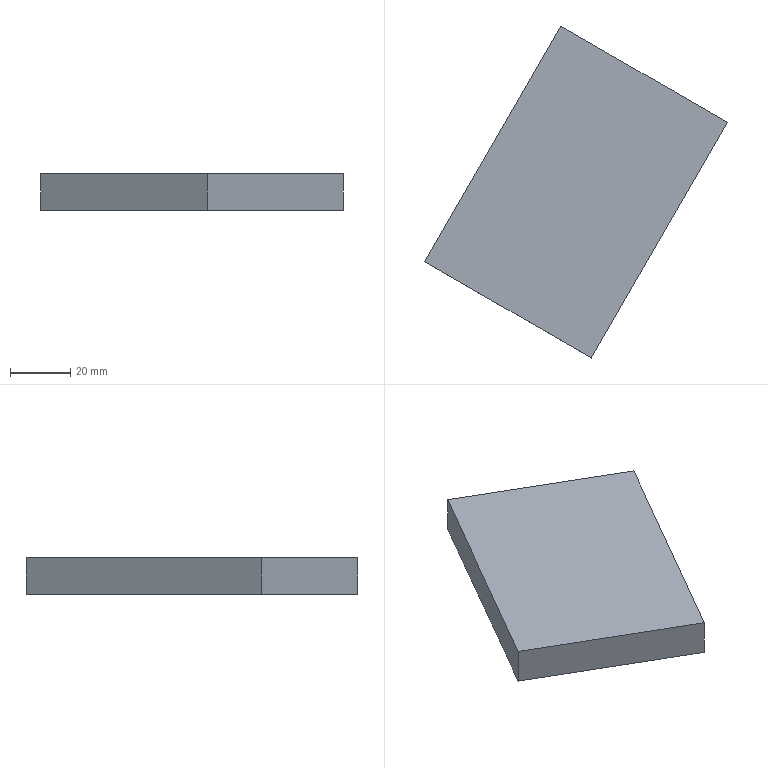Part | SolidWorks | features BaseBody 1 | 1 solid | 6 faces | box 100.197 x 109.81 x 12 mm | volume 68834 mm3 | plane 6
STEP:
#1=CARTESIAN_POINT('',(-225.308,1702.18,-1143.));
#2=VERTEX_POINT('',#1);
#3=CARTESIAN_POINT('',(-280.504,1734.048,-1143.));
#4=VERTEX_POINT('',#3);
#5=CARTESIAN_POINT('',(-225.308,1702.18,-1143.));
#6=DIRECTION('',(-0.866,0.5,0.));
#7=VECTOR('',#6,1000.);
#8=LINE('',#5,#7);
#9=EDGE_CURVE('',#2,#4,#8,.T.);
#10=ORIENTED_EDGE('',*,*,#9,.F.);
#11=CARTESIAN_POINT('',(-180.308,1780.122,-1143.));
#12=VERTEX_POINT('',#11);
#13=CARTESIAN_POINT('',(-180.308,1780.122,-1143.));
#14=DIRECTION('',(-0.5,-0.866,0.));
#15=VECTOR('',#14,1000.);
#16=LINE('',#13,#15);
#17=EDGE_CURVE('',#12,#2,#16,.T.);
#18=ORIENTED_EDGE('',*,*,#17,.F.);
#19=CARTESIAN_POINT('',(-235.504,1811.99,-1143.));
#20=VERTEX_POINT('',#19);
#21=CARTESIAN_POINT('',(-235.504,1811.99,-1143.));
#22=DIRECTION('',(0.866,-0.5,0.));
#23=VECTOR('',#22,1000.);
#24=LINE('',#21,#23);
#25=EDGE_CURVE('',#20,#12,#24,.T.);
#26=ORIENTED_EDGE('',*,*,#25,.F.);
#27=CARTESIAN_POINT('',(-280.504,1734.048,-1143.));
#28=DIRECTION('',(0.5,0.866,0.));
#29=VECTOR('',#28,1000.);
#30=LINE('',#27,#29);
#31=EDGE_CURVE('',#4,#20,#30,.T.);
#32=ORIENTED_EDGE('',*,*,#31,.F.);
#33=EDGE_LOOP('',(#10,#18,#26,#32));
#34=FACE_OUTER_BOUND('',#33,.T.);
#35=CARTESIAN_POINT('',(-240.684,1763.019,-1143.));
#36=DIRECTION('',(0.,0.,-1.));
#37=DIRECTION('',(-1.,0.,0.));
#38=AXIS2_PLACEMENT_3D('',#35,#36,#37);
#39=PLANE('',#38);
#40=ADVANCED_FACE('',(#34),#39,.F.);
#41=CARTESIAN_POINT('',(-280.504,1734.048,-1155.));
#42=VERTEX_POINT('',#41);
#43=CARTESIAN_POINT('',(-235.504,1811.99,-1155.));
#44=VERTEX_POINT('',#43);
#45=CARTESIAN_POINT('',(-280.504,1734.048,-1155.));
#46=DIRECTION('',(0.5,0.866,0.));
#47=VECTOR('',#46,1000.);
#48=LINE('',#45,#47);
#49=EDGE_CURVE('',#42,#44,#48,.T.);
#50=ORIENTED_EDGE('',*,*,#49,.F.);
#51=CARTESIAN_POINT('',(-280.504,1734.048,-1155.));
#52=DIRECTION('',(0.,0.,-1.));
#53=VECTOR('',#52,1000.);
#54=LINE('',#51,#53);
#55=EDGE_CURVE('',#4,#42,#54,.T.);
#56=ORIENTED_EDGE('',*,*,#55,.F.);
#57=ORIENTED_EDGE('',*,*,#31,.T.);
#58=CARTESIAN_POINT('',(-235.504,1811.99,-1155.));
#59=DIRECTION('',(0.,0.,1.));
#60=VECTOR('',#59,1000.);
#61=LINE('',#58,#60);
#62=EDGE_CURVE('',#44,#20,#61,.T.);
#63=ORIENTED_EDGE('',*,*,#62,.F.);
#64=EDGE_LOOP('',(#50,#56,#57,#63));
#65=FACE_OUTER_BOUND('',#64,.T.);
#66=CARTESIAN_POINT('',(-280.504,1734.048,-1155.));
#67=DIRECTION('',(0.866,-0.5,0.));
#68=DIRECTION('',(0.5,0.866,0.));
#69=AXIS2_PLACEMENT_3D('',#66,#67,#68);
#70=PLANE('',#69);
#71=ADVANCED_FACE('',(#65),#70,.F.);
#72=CARTESIAN_POINT('',(-225.308,1702.18,-1155.));
#73=VERTEX_POINT('',#72);
#74=CARTESIAN_POINT('',(-245.863,1714.048,-1155.));
#75=DIRECTION('',(-0.866,0.5,0.));
#76=VECTOR('',#75,1000.);
#77=LINE('',#74,#76);
#78=EDGE_CURVE('',#73,#42,#77,.T.);
#79=ORIENTED_EDGE('',*,*,#78,.F.);
#80=CARTESIAN_POINT('',(-225.308,1702.18,-1155.));
#81=DIRECTION('',(0.,0.,-1.));
#82=VECTOR('',#81,1000.);
#83=LINE('',#80,#82);
#84=EDGE_CURVE('',#2,#73,#83,.T.);
#85=ORIENTED_EDGE('',*,*,#84,.F.);
#86=ORIENTED_EDGE('',*,*,#9,.T.);
#87=ORIENTED_EDGE('',*,*,#55,.T.);
#88=EDGE_LOOP('',(#79,#85,#86,#87));
#89=FACE_OUTER_BOUND('',#88,.T.);
#90=CARTESIAN_POINT('',(-245.863,1714.048,-1155.));
#91=DIRECTION('',(0.5,0.866,0.));
#92=DIRECTION('',(-0.866,0.5,0.));
#93=AXIS2_PLACEMENT_3D('',#90,#91,#92);
#94=PLANE('',#93);
#95=ADVANCED_FACE('',(#89),#94,.F.);
#96=CARTESIAN_POINT('',(-180.308,1780.122,-1155.));
#97=VERTEX_POINT('',#96);
#98=CARTESIAN_POINT('',(-190.308,1762.802,-1155.));
#99=DIRECTION('',(-0.5,-0.866,0.));
#100=VECTOR('',#99,1000.);
#101=LINE('',#98,#100);
#102=EDGE_CURVE('',#97,#73,#101,.T.);
#103=ORIENTED_EDGE('',*,*,#102,.F.);
#104=CARTESIAN_POINT('',(-180.308,1780.122,-543.));
#105=DIRECTION('',(0.,0.,-1.));
#106=VECTOR('',#105,1000.);
#107=LINE('',#104,#106);
#108=EDGE_CURVE('',#12,#97,#107,.T.);
#109=ORIENTED_EDGE('',*,*,#108,.F.);
#110=ORIENTED_EDGE('',*,*,#17,.T.);
#111=ORIENTED_EDGE('',*,*,#84,.T.);
#112=EDGE_LOOP('',(#103,#109,#110,#111));
#113=FACE_OUTER_BOUND('',#112,.T.);
#114=CARTESIAN_POINT('',(-190.308,1762.802,-543.));
#115=DIRECTION('',(-0.866,0.5,0.));
#116=DIRECTION('',(-0.5,-0.866,0.));
#117=AXIS2_PLACEMENT_3D('',#114,#115,#116);
#118=PLANE('',#117);
#119=ADVANCED_FACE('',(#113),#118,.F.);
#120=CARTESIAN_POINT('',(-200.863,1791.99,-1155.));
#121=DIRECTION('',(0.866,-0.5,0.));
#122=VECTOR('',#121,1000.);
#123=LINE('',#120,#122);
#124=EDGE_CURVE('',#44,#97,#123,.T.);
#125=ORIENTED_EDGE('',*,*,#124,.F.);
#126=ORIENTED_EDGE('',*,*,#62,.T.);
#127=ORIENTED_EDGE('',*,*,#25,.T.);
#128=ORIENTED_EDGE('',*,*,#108,.T.);
#129=EDGE_LOOP('',(#125,#126,#127,#128));
#130=FACE_OUTER_BOUND('',#129,.T.);
#131=CARTESIAN_POINT('',(-200.863,1791.99,-1155.));
#132=DIRECTION('',(-0.5,-0.866,0.));
#133=DIRECTION('',(0.866,-0.5,0.));
#134=AXIS2_PLACEMENT_3D('',#131,#132,#133);
#135=PLANE('',#134);
#136=ADVANCED_FACE('',(#130),#135,.F.);
#137=ORIENTED_EDGE('',*,*,#49,.T.);
#138=ORIENTED_EDGE('',*,*,#124,.T.);
#139=ORIENTED_EDGE('',*,*,#102,.T.);
#140=ORIENTED_EDGE('',*,*,#78,.T.);
#141=EDGE_LOOP('',(#137,#138,#139,#140));
#142=FACE_OUTER_BOUND('',#141,.T.);
#143=CARTESIAN_POINT('',(-240.684,1763.019,-1155.));
#144=DIRECTION('',(0.,0.,-1.));
#145=DIRECTION('',(-1.,0.,0.));
#146=AXIS2_PLACEMENT_3D('',#143,#144,#145);
#147=PLANE('',#146);
#148=ADVANCED_FACE('',(#142),#147,.T.);
#149=CLOSED_SHELL('',(#40,#71,#95,#119,#136,#148));
#150=MANIFOLD_SOLID_BREP('',#149);
#151=CARTESIAN_POINT('',(0.,0.,0.));
#152=DIRECTION('',(0.,0.,1.));
#153=DIRECTION('',(1.,0.,0.));
#154=AXIS2_PLACEMENT_3D('',#151,#152,#153);
#155=(LENGTH_UNIT()NAMED_UNIT(*)SI_UNIT(.MILLI.,.METRE.));
#156=UNCERTAINTY_MEASURE_WITH_UNIT(LENGTH_MEASURE(0.00001),#155,'','');
#157=(NAMED_UNIT(*)PLANE_ANGLE_UNIT()SI_UNIT($,.RADIAN.));
#158=(NAMED_UNIT(*)SI_UNIT($,.STERADIAN.)SOLID_ANGLE_UNIT());
#159=(GEOMETRIC_REPRESENTATION_CONTEXT(3)GLOBAL_UNCERTAINTY_ASSIGNED_CONTEXT((#156))GLOBAL_UNIT_ASSIGNED_CONTEXT((#155,#157,#158))REPRESENTATION_CONTEXT('',''));
#160=ADVANCED_BREP_SHAPE_REPRESENTATION('',(#150,#154),#159);